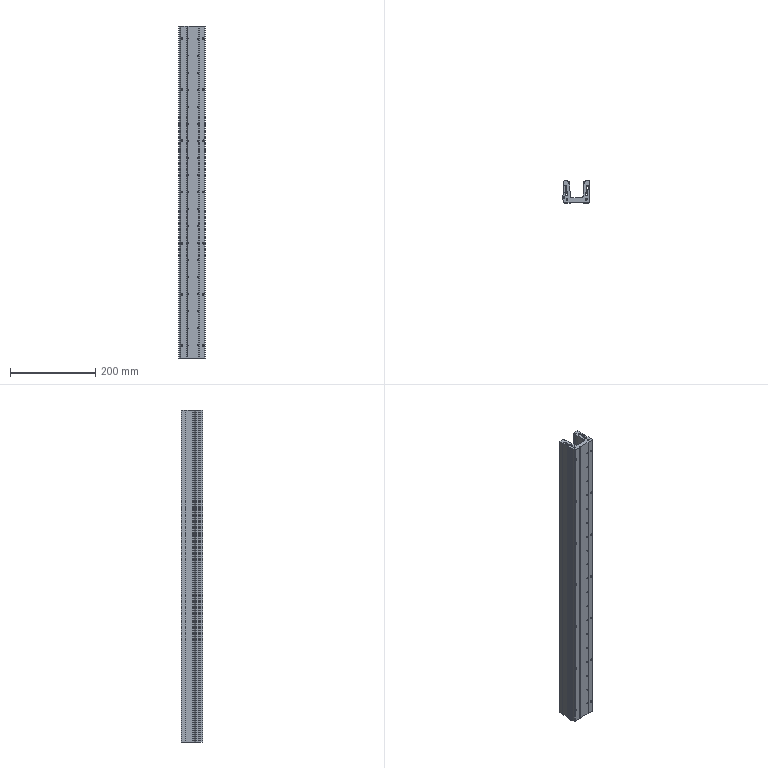Part | STEP file | BODY1_E-RAM6-S-640-ME30-C5 | 1 solid | 453 faces | box 63 x 51 x 780 mm | volume 1225538 mm3 | cylinder 241 | plane 158 | cone 54 | commonest cylinder face diameters 2 x102 7.5 x42 2.459 x38 1 x24 4.5 x14 0.6 x13